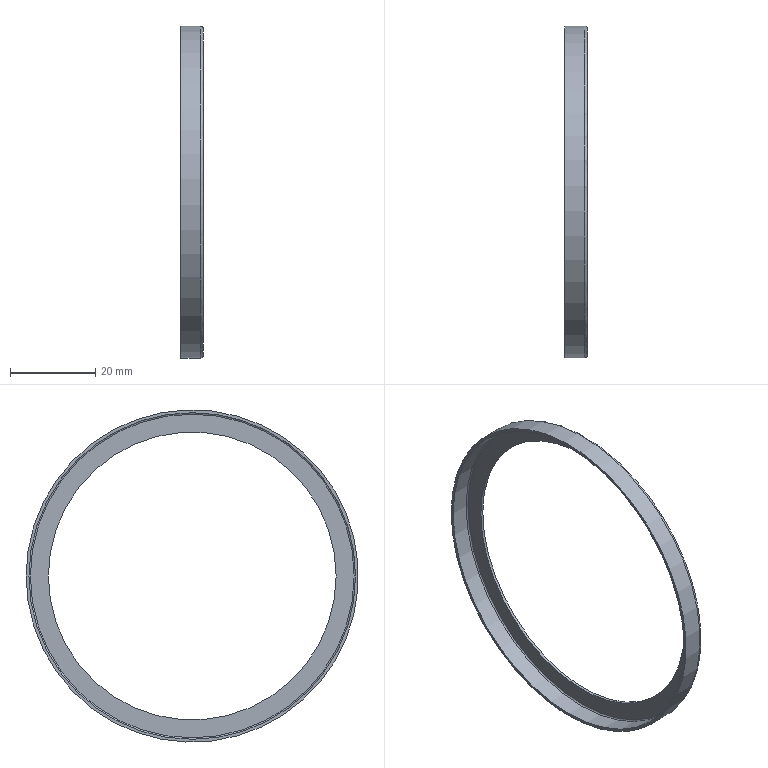Part | STEP file | Valve | 1 solid | 8 faces | box 5.28 x 77.925 x 77.925 mm | volume 1517 mm3 | cylinder 3 | plane 3 | torus 2 | commonest cylinder face diameters 67.5 x1 76.597 x1 77.925 x1
STEP:
#1=CARTESIAN_POINT('',(5.976,38.962,0.));
#2=VERTEX_POINT('',#1);
#3=CARTESIAN_POINT('',(5.976,0.,0.));
#4=DIRECTION('',(1.,0.,0.));
#5=DIRECTION('',(0.,1.,0.));
#6=AXIS2_PLACEMENT_3D('',#3,#4,#5);
#7=CIRCLE('',#6,38.962);
#8=EDGE_CURVE('',#2,#2,#7,.T.);
#9=ORIENTED_EDGE('',*,*,#8,.F.);
#10=EDGE_LOOP('',(#9));
#11=FACE_OUTER_BOUND('',#10,.T.);
#12=CARTESIAN_POINT('',(1.36,38.962,0.));
#13=VERTEX_POINT('',#12);
#14=CARTESIAN_POINT('',(1.36,0.,0.));
#15=DIRECTION('',(1.,0.,0.));
#16=DIRECTION('',(0.,1.,0.));
#17=AXIS2_PLACEMENT_3D('',#14,#15,#16);
#18=CIRCLE('',#17,38.962);
#19=EDGE_CURVE('',#13,#13,#18,.T.);
#20=ORIENTED_EDGE('',*,*,#19,.T.);
#21=EDGE_LOOP('',(#20));
#22=FACE_OUTER_BOUND('',#21,.T.);
#23=CARTESIAN_POINT('',(1.36,0.,0.));
#24=DIRECTION('',(1.,0.,0.));
#25=DIRECTION('',(0.,1.,0.));
#26=AXIS2_PLACEMENT_3D('',#23,#24,#25);
#27=CYLINDRICAL_SURFACE('',#26,38.962);
#28=ADVANCED_FACE('',(#11,#22),#27,.T.);
#29=ORIENTED_EDGE('',*,*,#19,.F.);
#30=EDGE_LOOP('',(#29));
#31=FACE_BOUND('',#30,.T.);
#32=CARTESIAN_POINT('',(1.36,38.298,0.));
#33=VERTEX_POINT('',#32);
#34=CARTESIAN_POINT('',(1.36,0.,0.));
#35=DIRECTION('',(1.,0.,0.));
#36=DIRECTION('',(0.,1.,0.));
#37=AXIS2_PLACEMENT_3D('',#34,#35,#36);
#38=CIRCLE('',#37,38.298);
#39=EDGE_CURVE('',#33,#33,#38,.T.);
#40=ORIENTED_EDGE('',*,*,#39,.T.);
#41=EDGE_LOOP('',(#40));
#42=FACE_BOUND('',#41,.T.);
#43=CARTESIAN_POINT('',(1.36,0.,0.));
#44=DIRECTION('',(-1.,0.,0.));
#45=DIRECTION('',(0.,1.,0.));
#46=AXIS2_PLACEMENT_3D('',#43,#44,#45);
#47=PLANE('',#46);
#48=ADVANCED_FACE('',(#31,#42),#47,.T.);
#49=CARTESIAN_POINT('',(5.644,38.298,0.));
#50=VERTEX_POINT('',#49);
#51=CARTESIAN_POINT('',(5.644,0.,0.));
#52=DIRECTION('',(1.,0.,0.));
#53=DIRECTION('',(0.,1.,0.));
#54=AXIS2_PLACEMENT_3D('',#51,#52,#53);
#55=CIRCLE('',#54,38.298);
#56=EDGE_CURVE('',#50,#50,#55,.T.);
#57=ORIENTED_EDGE('',*,*,#56,.T.);
#58=EDGE_LOOP('',(#57));
#59=FACE_OUTER_BOUND('',#58,.T.);
#60=ORIENTED_EDGE('',*,*,#39,.F.);
#61=EDGE_LOOP('',(#60));
#62=FACE_OUTER_BOUND('',#61,.T.);
#63=CARTESIAN_POINT('',(5.976,0.,0.));
#64=DIRECTION('',(1.,0.,0.));
#65=DIRECTION('',(0.,1.,0.));
#66=AXIS2_PLACEMENT_3D('',#63,#64,#65);
#67=CYLINDRICAL_SURFACE('',#66,38.298);
#68=ADVANCED_FACE('',(#59,#62),#67,.F.);
#69=CARTESIAN_POINT('',(5.976,37.967,0.));
#70=VERTEX_POINT('',#69);
#71=CARTESIAN_POINT('',(5.976,0.,0.));
#72=DIRECTION('',(1.,0.,0.));
#73=DIRECTION('',(0.,1.,0.));
#74=AXIS2_PLACEMENT_3D('',#71,#72,#73);
#75=CIRCLE('',#74,37.967);
#76=EDGE_CURVE('',#70,#70,#75,.T.);
#77=ORIENTED_EDGE('',*,*,#76,.F.);
#78=EDGE_LOOP('',(#77));
#79=FACE_BOUND('',#78,.T.);
#80=CARTESIAN_POINT('',(5.976,33.75,0.));
#81=VERTEX_POINT('',#80);
#82=CARTESIAN_POINT('',(5.976,0.,0.));
#83=DIRECTION('',(1.,0.,0.));
#84=DIRECTION('',(0.,1.,0.));
#85=AXIS2_PLACEMENT_3D('',#82,#83,#84);
#86=CIRCLE('',#85,33.75);
#87=EDGE_CURVE('',#81,#81,#86,.T.);
#88=ORIENTED_EDGE('',*,*,#87,.T.);
#89=EDGE_LOOP('',(#88));
#90=FACE_BOUND('',#89,.T.);
#91=CARTESIAN_POINT('',(5.976,0.,0.));
#92=DIRECTION('',(-1.,0.,0.));
#93=DIRECTION('',(0.,1.,0.));
#94=AXIS2_PLACEMENT_3D('',#91,#92,#93);
#95=PLANE('',#94);
#96=ADVANCED_FACE('',(#79,#90),#95,.T.);
#97=CARTESIAN_POINT('',(6.64,33.75,0.));
#98=VERTEX_POINT('',#97);
#99=CARTESIAN_POINT('',(6.64,0.,0.));
#100=DIRECTION('',(1.,0.,0.));
#101=DIRECTION('',(0.,1.,0.));
#102=AXIS2_PLACEMENT_3D('',#99,#100,#101);
#103=CIRCLE('',#102,33.75);
#104=EDGE_CURVE('',#98,#98,#103,.T.);
#105=ORIENTED_EDGE('',*,*,#104,.T.);
#106=EDGE_LOOP('',(#105));
#107=FACE_OUTER_BOUND('',#106,.T.);
#108=ORIENTED_EDGE('',*,*,#87,.F.);
#109=EDGE_LOOP('',(#108));
#110=FACE_OUTER_BOUND('',#109,.T.);
#111=CARTESIAN_POINT('',(6.64,0.,0.));
#112=DIRECTION('',(1.,0.,0.));
#113=DIRECTION('',(0.,1.,0.));
#114=AXIS2_PLACEMENT_3D('',#111,#112,#113);
#115=CYLINDRICAL_SURFACE('',#114,33.75);
#116=ADVANCED_FACE('',(#107,#110),#115,.F.);
#117=CARTESIAN_POINT('',(6.64,38.298,0.));
#118=VERTEX_POINT('',#117);
#119=CARTESIAN_POINT('',(6.64,0.,0.));
#120=DIRECTION('',(1.,0.,0.));
#121=DIRECTION('',(0.,1.,0.));
#122=AXIS2_PLACEMENT_3D('',#119,#120,#121);
#123=CIRCLE('',#122,38.298);
#124=EDGE_CURVE('',#118,#118,#123,.T.);
#125=ORIENTED_EDGE('',*,*,#124,.T.);
#126=EDGE_LOOP('',(#125));
#127=FACE_BOUND('',#126,.T.);
#128=ORIENTED_EDGE('',*,*,#104,.F.);
#129=EDGE_LOOP('',(#128));
#130=FACE_BOUND('',#129,.T.);
#131=CARTESIAN_POINT('',(6.64,0.,0.));
#132=DIRECTION('',(1.,0.,0.));
#133=DIRECTION('',(0.,1.,0.));
#134=AXIS2_PLACEMENT_3D('',#131,#132,#133);
#135=PLANE('',#134);
#136=ADVANCED_FACE('',(#127,#130),#135,.T.);
#137=ORIENTED_EDGE('',*,*,#124,.F.);
#138=EDGE_LOOP('',(#137));
#139=FACE_OUTER_BOUND('',#138,.T.);
#140=ORIENTED_EDGE('',*,*,#8,.T.);
#141=EDGE_LOOP('',(#140));
#142=FACE_OUTER_BOUND('',#141,.T.);
#143=CARTESIAN_POINT('',(5.976,0.,0.));
#144=DIRECTION('',(1.,0.,0.));
#145=DIRECTION('',(0.,1.,0.));
#146=AXIS2_PLACEMENT_3D('',#143,#144,#145);
#147=TOROIDAL_SURFACE('',#146,38.298,0.664);
#148=ADVANCED_FACE('',(#139,#142),#147,.T.);
#149=ORIENTED_EDGE('',*,*,#76,.T.);
#150=EDGE_LOOP('',(#149));
#151=FACE_OUTER_BOUND('',#150,.T.);
#152=ORIENTED_EDGE('',*,*,#56,.F.);
#153=EDGE_LOOP('',(#152));
#154=FACE_OUTER_BOUND('',#153,.T.);
#155=CARTESIAN_POINT('',(5.644,0.,0.));
#156=DIRECTION('',(1.,0.,0.));
#157=DIRECTION('',(0.,1.,0.));
#158=AXIS2_PLACEMENT_3D('',#155,#156,#157);
#159=TOROIDAL_SURFACE('',#158,37.967,0.332);
#160=ADVANCED_FACE('',(#151,#154),#159,.F.);
#161=CLOSED_SHELL('',(#28,#48,#68,#96,#116,#136,#148,#160));
#162=MANIFOLD_SOLID_BREP('',#161);
#163=(LENGTH_UNIT()NAMED_UNIT(*)SI_UNIT(.MILLI.,.METRE.));
#164=UNCERTAINTY_MEASURE_WITH_UNIT(LENGTH_MEASURE(0.00001),#163,'','');
#165=(NAMED_UNIT(*)PLANE_ANGLE_UNIT()SI_UNIT($,.RADIAN.));
#166=(NAMED_UNIT(*)SI_UNIT($,.STERADIAN.)SOLID_ANGLE_UNIT());
#167=(GEOMETRIC_REPRESENTATION_CONTEXT(3)GLOBAL_UNCERTAINTY_ASSIGNED_CONTEXT((#164))GLOBAL_UNIT_ASSIGNED_CONTEXT((#163,#165,#166))REPRESENTATION_CONTEXT('',''));
#168=ADVANCED_BREP_SHAPE_REPRESENTATION('',(#162),#167);